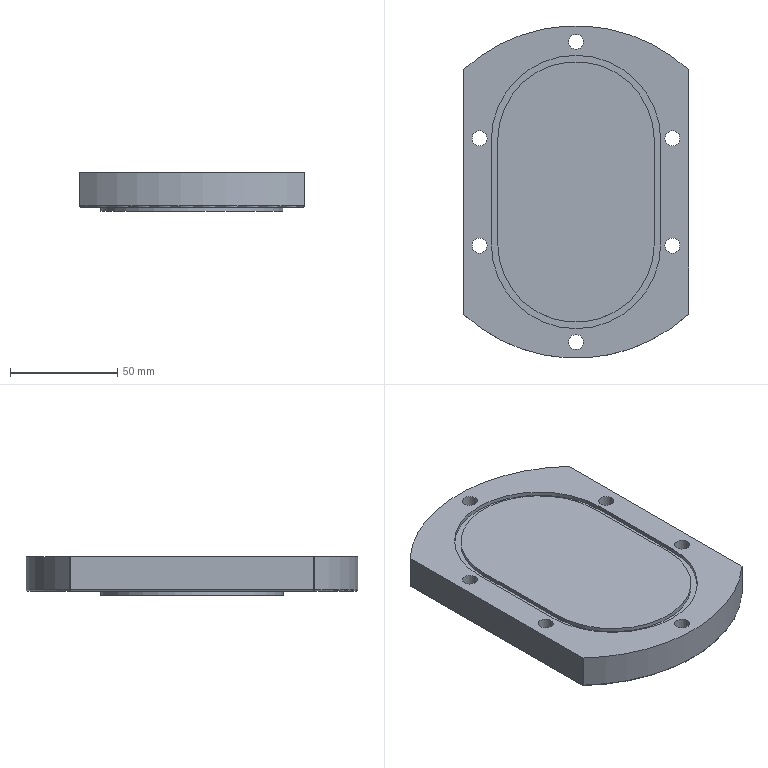CAM job | NX | 3-axis milling, drilling | part box 105 x 155 x 18 mm | stock box 105 x 155 x 23 mm
Tools:
number,name,description,diameter,corner_radius,flute_length,length,flutes
2,D50,Milling Tool-5 Parameters,50.0,0.0,50.0,75.0,2
1,ZXZ,Milling Tool-5 Parameters,6.0,0.0,50.0,75.0,2
9,7.0ZT,Drilling Tool,7.0,0.0,35.0,50.0,2
3,D3,Milling Tool-5 Parameters,3.0,0.0,50.0,75.0,2
5,D25R0.5,Milling Tool-5 Parameters,25.0,0.5,50.0,75.0,2
11,D10JING,Milling Tool-5 Parameters,10.0,0.0,50.0,75.0,2
7,D6A45,Milling Tool-5 Parameters,6.0,0.0,50.0,75.0,2
6,D6,Milling Tool-5 Parameters,6.0,0.0,50.0,75.0,2
Operations:
program,operation,operation_type,tool,method,geometry_group,spindle_rpm,surface_speed,feed_per_tooth,feed_cut,feed_plunge,cut_length_mm,path_length_mm,cut_time_min,machine_time_min
1,FLOOR_WALL_COPY_1,VolumeBased25DMillingOperation,D50,METHOD,A,1200.0,188.0,0.8333,2000.0,1000.0,16145.523,19817.896,8.126,8.494
1,FLOOR_WALL_COPY_COPY,VolumeBased25DMillingOperation,D50,METHOD,A,2500.0,392.0,0.2,1000.0,1000.0,1153.241,1207.241,1.153,1.159
1,DRILLING,Operation,ZXZ,METHOD,A,5000.0,94.0,0.025,250.0,0.0,24.0,414.311,0.096,0.135
1,DRILLING_COPY,Operation,7.0ZT,METHOD,A,2000.0,59.0,0.05,200.0,0.0,144.618,721.847,0.7231,0.7808
1,PLANAR_PROFILE,PlanarMilling,D3,METHOD,A,5000.0,47.0,0.11,1100.0,500.0,12305.198,12360.997,11.306,11.312
1,ZLEVEL_PROFILE_COPY,ZLevelMilling,D25R0.5,METHOD,A,2000.0,157.0,0.55,2200.0,1000.0,12915.404,24949.625,6.454,11.818
1,ZLEVEL_PROFILE_1,ZLevelMilling,D10JING,METHOD,A,5000.0,157.0,0.125,1250.0,100.0,253.216,547.891,0.2026,0.232
1,PLANAR_MILL_COPY_COPY,PlanarMilling,D6A45,METHOD,A,7500.0,141.0,0.0833,1250.0,100.0,1291.012,2182.452,1.033,1.122
2,FLOOR_WALL_COPY_1_COPY,VolumeBased25DMillingOperation,D50,METHOD,B,1200.0,188.0,0.8333,2000.0,1000.0,9258.215,11064.825,4.678,4.859
2,FLOOR_WALL_COPY_COPY_COPY,VolumeBased25DMillingOperation,D50,METHOD,B,2500.0,392.0,0.2,1000.0,1000.0,661.301,715.301,0.6613,0.6667
2,HOLE_MILLING_COPY_COPY,CylinderMilling,D6,METHOD,B,4987.0,94.0,0.1504,1500.0,100.0,7492.847,8257.685,4.995,5.072
2,PLANAR_MILL_COPY_COPY_COPY,PlanarMilling,D6A45,METHOD,B,7500.0,141.0,0.0833,1250.0,100.0,282.949,339.949,0.2264,0.2321
2,PLANAR_MILL_COPY_COPY_COPY_COPY,PlanarMilling,D6A45,METHOD,B,7500.0,141.0,0.0833,1250.0,100.0,679.398,1476.467,0.5435,0.6232